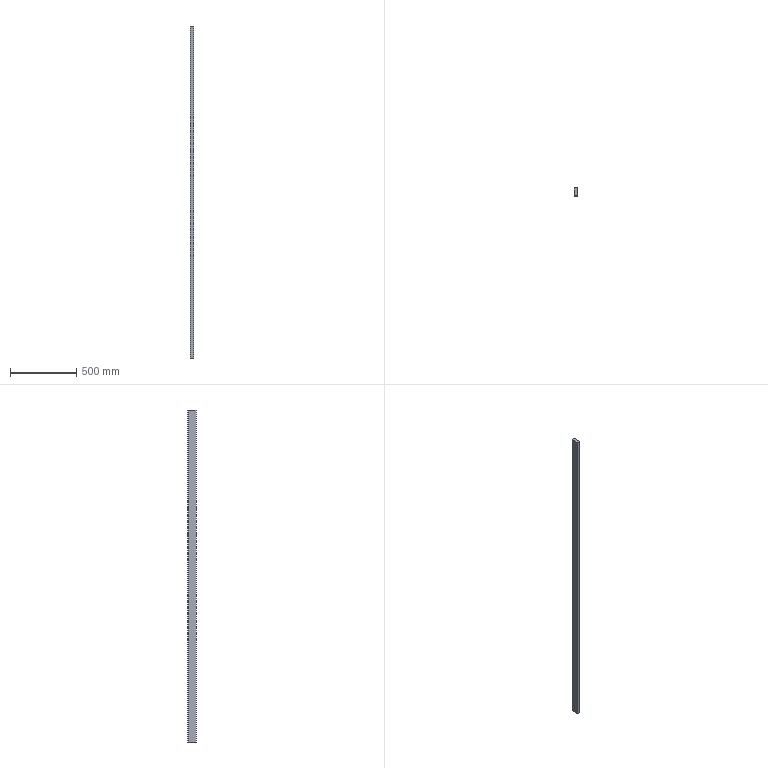Part | STEP file | Part 16 | 1 solid | 8 faces | box 25 x 62 x 2500 mm | volume 3760000 mm3 | plane 8
STEP:
#1=CARTESIAN_POINT('',(13.5,-60.,-2500.));
#2=VERTEX_POINT('',#1);
#3=CARTESIAN_POINT('',(13.5,2.,-2500.));
#4=VERTEX_POINT('',#3);
#5=CARTESIAN_POINT('',(13.5,-60.,-2500.));
#6=DIRECTION('',(0.,1.,0.));
#7=VECTOR('',#6,1000.);
#8=LINE('',#5,#7);
#9=EDGE_CURVE('',#2,#4,#8,.T.);
#10=ORIENTED_EDGE('',*,*,#9,.F.);
#11=CARTESIAN_POINT('',(-11.5,-60.,-2500.));
#12=VERTEX_POINT('',#11);
#13=CARTESIAN_POINT('',(-11.5,-60.,-2500.));
#14=DIRECTION('',(1.,0.,0.));
#15=VECTOR('',#14,1000.);
#16=LINE('',#13,#15);
#17=EDGE_CURVE('',#12,#2,#16,.T.);
#18=ORIENTED_EDGE('',*,*,#17,.F.);
#19=CARTESIAN_POINT('',(-11.5,0.,-2500.));
#20=VERTEX_POINT('',#19);
#21=CARTESIAN_POINT('',(-11.5,0.,-2500.));
#22=DIRECTION('',(0.,-1.,0.));
#23=VECTOR('',#22,1000.);
#24=LINE('',#21,#23);
#25=EDGE_CURVE('',#20,#12,#24,.T.);
#26=ORIENTED_EDGE('',*,*,#25,.F.);
#27=CARTESIAN_POINT('',(11.5,0.,-2500.));
#28=VERTEX_POINT('',#27);
#29=CARTESIAN_POINT('',(11.5,0.,-2500.));
#30=DIRECTION('',(-1.,0.,0.));
#31=VECTOR('',#30,1000.);
#32=LINE('',#29,#31);
#33=EDGE_CURVE('',#28,#20,#32,.T.);
#34=ORIENTED_EDGE('',*,*,#33,.F.);
#35=CARTESIAN_POINT('',(11.5,2.,-2500.));
#36=VERTEX_POINT('',#35);
#37=CARTESIAN_POINT('',(11.5,2.,-2500.));
#38=DIRECTION('',(0.,-1.,0.));
#39=VECTOR('',#38,1000.);
#40=LINE('',#37,#39);
#41=EDGE_CURVE('',#36,#28,#40,.T.);
#42=ORIENTED_EDGE('',*,*,#41,.F.);
#43=CARTESIAN_POINT('',(13.5,2.,-2500.));
#44=DIRECTION('',(-1.,0.,0.));
#45=VECTOR('',#44,1000.);
#46=LINE('',#43,#45);
#47=EDGE_CURVE('',#4,#36,#46,.T.);
#48=ORIENTED_EDGE('',*,*,#47,.F.);
#49=EDGE_LOOP('',(#10,#18,#26,#34,#42,#48));
#50=FACE_OUTER_BOUND('',#49,.T.);
#51=CARTESIAN_POINT('',(-10.995,12.455,-2500.));
#52=DIRECTION('',(0.,0.,-1.));
#53=DIRECTION('',(-1.,0.,0.));
#54=AXIS2_PLACEMENT_3D('',#51,#52,#53);
#55=PLANE('',#54);
#56=ADVANCED_FACE('',(#50),#55,.T.);
#57=CARTESIAN_POINT('',(13.5,-60.,0.));
#58=VERTEX_POINT('',#57);
#59=CARTESIAN_POINT('',(13.5,2.,0.));
#60=VERTEX_POINT('',#59);
#61=CARTESIAN_POINT('',(13.5,-60.,0.));
#62=DIRECTION('',(0.,1.,0.));
#63=VECTOR('',#62,1000.);
#64=LINE('',#61,#63);
#65=EDGE_CURVE('',#58,#60,#64,.T.);
#66=ORIENTED_EDGE('',*,*,#65,.T.);
#67=CARTESIAN_POINT('',(11.5,2.,0.));
#68=VERTEX_POINT('',#67);
#69=CARTESIAN_POINT('',(13.5,2.,0.));
#70=DIRECTION('',(-1.,0.,0.));
#71=VECTOR('',#70,1000.);
#72=LINE('',#69,#71);
#73=EDGE_CURVE('',#60,#68,#72,.T.);
#74=ORIENTED_EDGE('',*,*,#73,.T.);
#75=CARTESIAN_POINT('',(11.5,0.,0.));
#76=VERTEX_POINT('',#75);
#77=CARTESIAN_POINT('',(11.5,2.,0.));
#78=DIRECTION('',(0.,-1.,0.));
#79=VECTOR('',#78,1000.);
#80=LINE('',#77,#79);
#81=EDGE_CURVE('',#68,#76,#80,.T.);
#82=ORIENTED_EDGE('',*,*,#81,.T.);
#83=CARTESIAN_POINT('',(-11.5,0.,0.));
#84=VERTEX_POINT('',#83);
#85=CARTESIAN_POINT('',(11.5,0.,0.));
#86=DIRECTION('',(-1.,0.,0.));
#87=VECTOR('',#86,1000.);
#88=LINE('',#85,#87);
#89=EDGE_CURVE('',#76,#84,#88,.T.);
#90=ORIENTED_EDGE('',*,*,#89,.T.);
#91=CARTESIAN_POINT('',(-11.5,-60.,0.));
#92=VERTEX_POINT('',#91);
#93=CARTESIAN_POINT('',(-11.5,0.,0.));
#94=DIRECTION('',(0.,-1.,0.));
#95=VECTOR('',#94,1000.);
#96=LINE('',#93,#95);
#97=EDGE_CURVE('',#84,#92,#96,.T.);
#98=ORIENTED_EDGE('',*,*,#97,.T.);
#99=CARTESIAN_POINT('',(-11.5,-60.,0.));
#100=DIRECTION('',(1.,0.,0.));
#101=VECTOR('',#100,1000.);
#102=LINE('',#99,#101);
#103=EDGE_CURVE('',#92,#58,#102,.T.);
#104=ORIENTED_EDGE('',*,*,#103,.T.);
#105=EDGE_LOOP('',(#66,#74,#82,#90,#98,#104));
#106=FACE_OUTER_BOUND('',#105,.T.);
#107=CARTESIAN_POINT('',(0.,0.,0.));
#108=DIRECTION('',(0.,0.,1.));
#109=DIRECTION('',(1.,0.,0.));
#110=AXIS2_PLACEMENT_3D('',#107,#108,#109);
#111=PLANE('',#110);
#112=ADVANCED_FACE('',(#106),#111,.T.);
#113=CARTESIAN_POINT('',(13.5,2.,-2566.851));
#114=DIRECTION('',(0.,0.,1.));
#115=VECTOR('',#114,1000.);
#116=LINE('',#113,#115);
#117=EDGE_CURVE('',#4,#60,#116,.T.);
#118=ORIENTED_EDGE('',*,*,#117,.F.);
#119=ORIENTED_EDGE('',*,*,#47,.T.);
#120=CARTESIAN_POINT('',(11.5,2.,-2566.851));
#121=DIRECTION('',(0.,0.,1.));
#122=VECTOR('',#121,1000.);
#123=LINE('',#120,#122);
#124=EDGE_CURVE('',#36,#68,#123,.T.);
#125=ORIENTED_EDGE('',*,*,#124,.T.);
#126=ORIENTED_EDGE('',*,*,#73,.F.);
#127=EDGE_LOOP('',(#118,#119,#125,#126));
#128=FACE_OUTER_BOUND('',#127,.T.);
#129=CARTESIAN_POINT('',(13.5,2.,-2566.851));
#130=DIRECTION('',(0.,1.,0.));
#131=DIRECTION('',(-1.,0.,0.));
#132=AXIS2_PLACEMENT_3D('',#129,#130,#131);
#133=PLANE('',#132);
#134=ADVANCED_FACE('',(#128),#133,.T.);
#135=ORIENTED_EDGE('',*,*,#124,.F.);
#136=ORIENTED_EDGE('',*,*,#41,.T.);
#137=CARTESIAN_POINT('',(11.5,0.,-2566.851));
#138=DIRECTION('',(0.,0.,1.));
#139=VECTOR('',#138,1000.);
#140=LINE('',#137,#139);
#141=EDGE_CURVE('',#28,#76,#140,.T.);
#142=ORIENTED_EDGE('',*,*,#141,.T.);
#143=ORIENTED_EDGE('',*,*,#81,.F.);
#144=EDGE_LOOP('',(#135,#136,#142,#143));
#145=FACE_OUTER_BOUND('',#144,.T.);
#146=CARTESIAN_POINT('',(11.5,2.,-2566.851));
#147=DIRECTION('',(-1.,0.,0.));
#148=DIRECTION('',(0.,0.,1.));
#149=AXIS2_PLACEMENT_3D('',#146,#147,#148);
#150=PLANE('',#149);
#151=ADVANCED_FACE('',(#145),#150,.T.);
#152=ORIENTED_EDGE('',*,*,#141,.F.);
#153=ORIENTED_EDGE('',*,*,#33,.T.);
#154=CARTESIAN_POINT('',(-11.5,0.,-2566.851));
#155=DIRECTION('',(0.,0.,1.));
#156=VECTOR('',#155,1000.);
#157=LINE('',#154,#156);
#158=EDGE_CURVE('',#20,#84,#157,.T.);
#159=ORIENTED_EDGE('',*,*,#158,.T.);
#160=ORIENTED_EDGE('',*,*,#89,.F.);
#161=EDGE_LOOP('',(#152,#153,#159,#160));
#162=FACE_OUTER_BOUND('',#161,.T.);
#163=CARTESIAN_POINT('',(11.5,0.,-2566.851));
#164=DIRECTION('',(0.,1.,0.));
#165=DIRECTION('',(-1.,0.,0.));
#166=AXIS2_PLACEMENT_3D('',#163,#164,#165);
#167=PLANE('',#166);
#168=ADVANCED_FACE('',(#162),#167,.T.);
#169=ORIENTED_EDGE('',*,*,#158,.F.);
#170=ORIENTED_EDGE('',*,*,#25,.T.);
#171=CARTESIAN_POINT('',(-11.5,-60.,-2566.851));
#172=DIRECTION('',(0.,0.,1.));
#173=VECTOR('',#172,1000.);
#174=LINE('',#171,#173);
#175=EDGE_CURVE('',#12,#92,#174,.T.);
#176=ORIENTED_EDGE('',*,*,#175,.T.);
#177=ORIENTED_EDGE('',*,*,#97,.F.);
#178=EDGE_LOOP('',(#169,#170,#176,#177));
#179=FACE_OUTER_BOUND('',#178,.T.);
#180=CARTESIAN_POINT('',(-11.5,0.,-2566.851));
#181=DIRECTION('',(-1.,0.,0.));
#182=DIRECTION('',(0.,-1.,0.));
#183=AXIS2_PLACEMENT_3D('',#180,#181,#182);
#184=PLANE('',#183);
#185=ADVANCED_FACE('',(#179),#184,.T.);
#186=ORIENTED_EDGE('',*,*,#175,.F.);
#187=ORIENTED_EDGE('',*,*,#17,.T.);
#188=CARTESIAN_POINT('',(13.5,-60.,-2566.851));
#189=DIRECTION('',(0.,0.,1.));
#190=VECTOR('',#189,1000.);
#191=LINE('',#188,#190);
#192=EDGE_CURVE('',#2,#58,#191,.T.);
#193=ORIENTED_EDGE('',*,*,#192,.T.);
#194=ORIENTED_EDGE('',*,*,#103,.F.);
#195=EDGE_LOOP('',(#186,#187,#193,#194));
#196=FACE_OUTER_BOUND('',#195,.T.);
#197=CARTESIAN_POINT('',(-11.5,-60.,-2566.851));
#198=DIRECTION('',(0.,-1.,0.));
#199=DIRECTION('',(1.,0.,0.));
#200=AXIS2_PLACEMENT_3D('',#197,#198,#199);
#201=PLANE('',#200);
#202=ADVANCED_FACE('',(#196),#201,.T.);
#203=ORIENTED_EDGE('',*,*,#192,.F.);
#204=ORIENTED_EDGE('',*,*,#9,.T.);
#205=ORIENTED_EDGE('',*,*,#117,.T.);
#206=ORIENTED_EDGE('',*,*,#65,.F.);
#207=EDGE_LOOP('',(#203,#204,#205,#206));
#208=FACE_OUTER_BOUND('',#207,.T.);
#209=CARTESIAN_POINT('',(13.5,-60.,-2566.851));
#210=DIRECTION('',(1.,0.,0.));
#211=DIRECTION('',(0.,1.,0.));
#212=AXIS2_PLACEMENT_3D('',#209,#210,#211);
#213=PLANE('',#212);
#214=ADVANCED_FACE('',(#208),#213,.T.);
#215=CLOSED_SHELL('',(#56,#112,#134,#151,#168,#185,#202,#214));
#216=MANIFOLD_SOLID_BREP('',#215);
#217=CARTESIAN_POINT('',(0.,0.,0.));
#218=DIRECTION('',(0.,0.,1.));
#219=DIRECTION('',(1.,0.,0.));
#220=AXIS2_PLACEMENT_3D('',#217,#218,#219);
#221=(LENGTH_UNIT()NAMED_UNIT(*)SI_UNIT(.MILLI.,.METRE.));
#222=UNCERTAINTY_MEASURE_WITH_UNIT(LENGTH_MEASURE(0.00001),#221,'','');
#223=(NAMED_UNIT(*)PLANE_ANGLE_UNIT()SI_UNIT($,.RADIAN.));
#224=(NAMED_UNIT(*)SI_UNIT($,.STERADIAN.)SOLID_ANGLE_UNIT());
#225=(GEOMETRIC_REPRESENTATION_CONTEXT(3)GLOBAL_UNCERTAINTY_ASSIGNED_CONTEXT((#222))GLOBAL_UNIT_ASSIGNED_CONTEXT((#221,#223,#224))REPRESENTATION_CONTEXT('',''));
#226=ADVANCED_BREP_SHAPE_REPRESENTATION('',(#216,#220),#225);